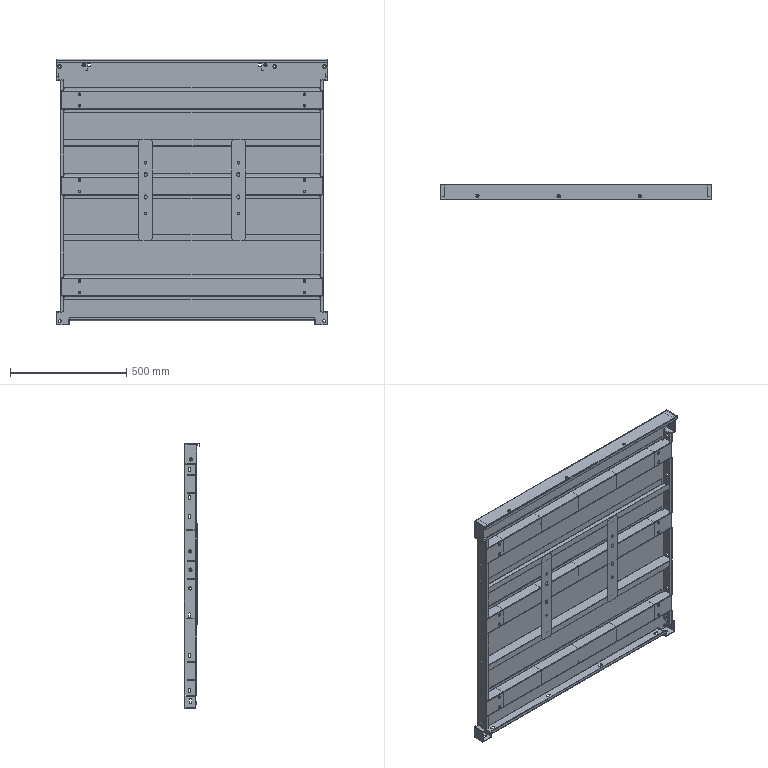Part | SolidWorks | features ReferencePattern 9, MirrorCompFeat 3, 3DProfileFeature 1, AEMSimFeature 1 | 55 solids | 1650 faces | box 1171 x 67 x 1143 mm | volume 7393142 mm3 | plane 1064 | cylinder 388 | cone 168 | spline 30 | commonest cylinder face diameters 6.917 x56 10.45 x56 10.77 x56 0.4 x40 6.4 x36 9 x36